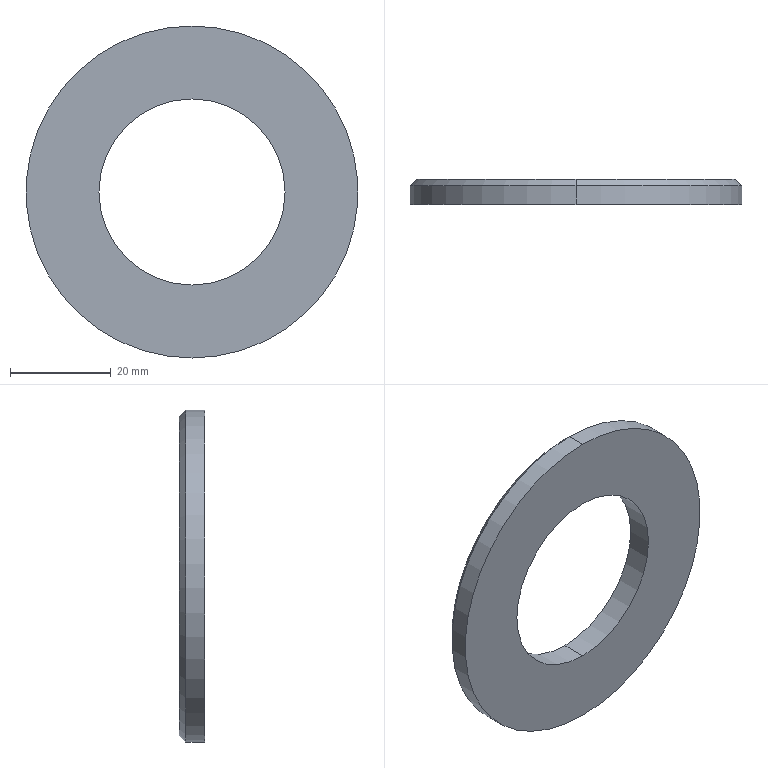Part | SolidWorks | features Revolution 1 | 1 solid | 8 faces | box 66 x 5 x 66 mm | volume 11570 mm3 | cylinder 4 | cone 2 | plane 2 | commonest cylinder face diameters 37 x2 66 x2
STEP:
#1=CARTESIAN_POINT('',(0.,12.395,-33.));
#2=VERTEX_POINT('',#1);
#3=CARTESIAN_POINT('',(0.,12.395,33.));
#4=VERTEX_POINT('',#3);
#5=CARTESIAN_POINT('',(0.,12.395,0.));
#6=DIRECTION('',(0.,-1.,0.));
#7=DIRECTION('',(0.,0.,-1.));
#8=AXIS2_PLACEMENT_3D('',#5,#6,#7);
#9=CIRCLE('',#8,33.);
#10=EDGE_CURVE('',#2,#4,#9,.T.);
#11=ORIENTED_EDGE('',*,*,#10,.T.);
#12=CARTESIAN_POINT('',(0.,8.645,33.));
#13=VERTEX_POINT('',#12);
#14=CARTESIAN_POINT('',(0.,0.,33.));
#15=DIRECTION('',(0.,-1.,0.));
#16=VECTOR('',#15,1000.);
#17=LINE('',#14,#16);
#18=EDGE_CURVE('',#4,#13,#17,.T.);
#19=ORIENTED_EDGE('',*,*,#18,.T.);
#20=CARTESIAN_POINT('',(0.,8.645,-33.));
#21=VERTEX_POINT('',#20);
#22=CARTESIAN_POINT('',(0.,8.645,0.));
#23=DIRECTION('',(0.,-1.,0.));
#24=DIRECTION('',(0.,0.,-1.));
#25=AXIS2_PLACEMENT_3D('',#22,#23,#24);
#26=CIRCLE('',#25,33.);
#27=EDGE_CURVE('',#21,#13,#26,.T.);
#28=ORIENTED_EDGE('',*,*,#27,.F.);
#29=CARTESIAN_POINT('',(0.,0.,-33.));
#30=DIRECTION('',(0.,-1.,0.));
#31=VECTOR('',#30,1000.);
#32=LINE('',#29,#31);
#33=EDGE_CURVE('',#2,#21,#32,.T.);
#34=ORIENTED_EDGE('',*,*,#33,.F.);
#35=EDGE_LOOP('',(#11,#19,#28,#34));
#36=FACE_OUTER_BOUND('',#35,.T.);
#37=CARTESIAN_POINT('',(0.,0.,0.));
#38=DIRECTION('',(0.,-1.,0.));
#39=DIRECTION('',(0.,0.,-1.));
#40=AXIS2_PLACEMENT_3D('',#37,#38,#39);
#41=CYLINDRICAL_SURFACE('',#40,33.);
#42=ADVANCED_FACE('',(#36),#41,.T.);
#43=CARTESIAN_POINT('',(0.,13.645,-31.75));
#44=VERTEX_POINT('',#43);
#45=CARTESIAN_POINT('',(0.,13.645,31.75));
#46=VERTEX_POINT('',#45);
#47=CARTESIAN_POINT('',(0.,13.645,0.));
#48=DIRECTION('',(0.,-1.,0.));
#49=DIRECTION('',(0.,0.,-1.));
#50=AXIS2_PLACEMENT_3D('',#47,#48,#49);
#51=CIRCLE('',#50,31.75);
#52=EDGE_CURVE('',#44,#46,#51,.T.);
#53=ORIENTED_EDGE('',*,*,#52,.T.);
#54=CARTESIAN_POINT('',(0.,13.645,31.75));
#55=DIRECTION('',(0.,-0.7071,0.7071));
#56=VECTOR('',#55,1000.);
#57=LINE('',#54,#56);
#58=EDGE_CURVE('',#46,#4,#57,.T.);
#59=ORIENTED_EDGE('',*,*,#58,.T.);
#60=ORIENTED_EDGE('',*,*,#10,.F.);
#61=CARTESIAN_POINT('',(0.,13.645,-31.75));
#62=DIRECTION('',(0.,-0.7071,-0.7071));
#63=VECTOR('',#62,1000.);
#64=LINE('',#61,#63);
#65=EDGE_CURVE('',#44,#2,#64,.T.);
#66=ORIENTED_EDGE('',*,*,#65,.F.);
#67=EDGE_LOOP('',(#53,#59,#60,#66));
#68=FACE_OUTER_BOUND('',#67,.T.);
#69=CARTESIAN_POINT('',(0.,13.645,0.));
#70=DIRECTION('',(0.,-1.,0.));
#71=DIRECTION('',(0.,0.,-1.));
#72=AXIS2_PLACEMENT_3D('',#69,#70,#71);
#73=CONICAL_SURFACE('',#72,31.75,0.7854);
#74=ADVANCED_FACE('',(#68),#73,.T.);
#75=CARTESIAN_POINT('',(0.,13.645,18.5));
#76=VERTEX_POINT('',#75);
#77=CARTESIAN_POINT('',(0.,13.645,-18.5));
#78=VERTEX_POINT('',#77);
#79=CARTESIAN_POINT('',(0.,13.645,0.));
#80=DIRECTION('',(0.,-1.,0.));
#81=DIRECTION('',(0.,0.,-1.));
#82=AXIS2_PLACEMENT_3D('',#79,#80,#81);
#83=CIRCLE('',#82,18.5);
#84=EDGE_CURVE('',#76,#78,#83,.T.);
#85=ORIENTED_EDGE('',*,*,#84,.F.);
#86=CARTESIAN_POINT('',(0.,8.645,18.5));
#87=VERTEX_POINT('',#86);
#88=CARTESIAN_POINT('',(0.,0.,18.5));
#89=DIRECTION('',(0.,-1.,0.));
#90=VECTOR('',#89,1000.);
#91=LINE('',#88,#90);
#92=EDGE_CURVE('',#76,#87,#91,.T.);
#93=ORIENTED_EDGE('',*,*,#92,.T.);
#94=CARTESIAN_POINT('',(0.,8.645,-18.5));
#95=VERTEX_POINT('',#94);
#96=CARTESIAN_POINT('',(0.,8.645,0.));
#97=DIRECTION('',(0.,-1.,0.));
#98=DIRECTION('',(0.,0.,-1.));
#99=AXIS2_PLACEMENT_3D('',#96,#97,#98);
#100=CIRCLE('',#99,18.5);
#101=EDGE_CURVE('',#87,#95,#100,.T.);
#102=ORIENTED_EDGE('',*,*,#101,.T.);
#103=CARTESIAN_POINT('',(0.,0.,-18.5));
#104=DIRECTION('',(0.,-1.,0.));
#105=VECTOR('',#104,1000.);
#106=LINE('',#103,#105);
#107=EDGE_CURVE('',#78,#95,#106,.T.);
#108=ORIENTED_EDGE('',*,*,#107,.F.);
#109=EDGE_LOOP('',(#85,#93,#102,#108));
#110=FACE_OUTER_BOUND('',#109,.T.);
#111=CARTESIAN_POINT('',(0.,0.,0.));
#112=DIRECTION('',(0.,-1.,0.));
#113=DIRECTION('',(0.,0.,-1.));
#114=AXIS2_PLACEMENT_3D('',#111,#112,#113);
#115=CYLINDRICAL_SURFACE('',#114,18.5);
#116=ADVANCED_FACE('',(#110),#115,.F.);
#117=ORIENTED_EDGE('',*,*,#92,.F.);
#118=CARTESIAN_POINT('',(0.,13.645,0.));
#119=DIRECTION('',(0.,-1.,0.));
#120=DIRECTION('',(0.,0.,-1.));
#121=AXIS2_PLACEMENT_3D('',#118,#119,#120);
#122=CIRCLE('',#121,18.5);
#123=EDGE_CURVE('',#78,#76,#122,.T.);
#124=ORIENTED_EDGE('',*,*,#123,.F.);
#125=ORIENTED_EDGE('',*,*,#107,.T.);
#126=CARTESIAN_POINT('',(0.,8.645,0.));
#127=DIRECTION('',(0.,-1.,0.));
#128=DIRECTION('',(0.,0.,-1.));
#129=AXIS2_PLACEMENT_3D('',#126,#127,#128);
#130=CIRCLE('',#129,18.5);
#131=EDGE_CURVE('',#95,#87,#130,.T.);
#132=ORIENTED_EDGE('',*,*,#131,.T.);
#133=EDGE_LOOP('',(#117,#124,#125,#132));
#134=FACE_OUTER_BOUND('',#133,.T.);
#135=CARTESIAN_POINT('',(0.,0.,0.));
#136=DIRECTION('',(0.,-1.,0.));
#137=DIRECTION('',(0.,0.,-1.));
#138=AXIS2_PLACEMENT_3D('',#135,#136,#137);
#139=CYLINDRICAL_SURFACE('',#138,18.5);
#140=ADVANCED_FACE('',(#134),#139,.F.);
#141=ORIENTED_EDGE('',*,*,#52,.F.);
#142=CARTESIAN_POINT('',(0.,13.645,0.));
#143=DIRECTION('',(0.,-1.,0.));
#144=DIRECTION('',(0.,0.,-1.));
#145=AXIS2_PLACEMENT_3D('',#142,#143,#144);
#146=CIRCLE('',#145,31.75);
#147=EDGE_CURVE('',#46,#44,#146,.T.);
#148=ORIENTED_EDGE('',*,*,#147,.F.);
#149=EDGE_LOOP('',(#141,#148));
#150=FACE_OUTER_BOUND('',#149,.T.);
#151=ORIENTED_EDGE('',*,*,#123,.T.);
#152=ORIENTED_EDGE('',*,*,#84,.T.);
#153=EDGE_LOOP('',(#151,#152));
#154=FACE_BOUND('',#153,.T.);
#155=CARTESIAN_POINT('',(-18.5,13.645,0.));
#156=DIRECTION('',(0.,-1.,0.));
#157=DIRECTION('',(0.,0.,-1.));
#158=AXIS2_PLACEMENT_3D('',#155,#156,#157);
#159=PLANE('',#158);
#160=ADVANCED_FACE('',(#150,#154),#159,.F.);
#161=ORIENTED_EDGE('',*,*,#58,.F.);
#162=ORIENTED_EDGE('',*,*,#147,.T.);
#163=ORIENTED_EDGE('',*,*,#65,.T.);
#164=CARTESIAN_POINT('',(0.,12.395,0.));
#165=DIRECTION('',(0.,-1.,0.));
#166=DIRECTION('',(0.,0.,-1.));
#167=AXIS2_PLACEMENT_3D('',#164,#165,#166);
#168=CIRCLE('',#167,33.);
#169=EDGE_CURVE('',#4,#2,#168,.T.);
#170=ORIENTED_EDGE('',*,*,#169,.F.);
#171=EDGE_LOOP('',(#161,#162,#163,#170));
#172=FACE_OUTER_BOUND('',#171,.T.);
#173=CARTESIAN_POINT('',(0.,13.645,0.));
#174=DIRECTION('',(0.,-1.,0.));
#175=DIRECTION('',(0.,0.,-1.));
#176=AXIS2_PLACEMENT_3D('',#173,#174,#175);
#177=CONICAL_SURFACE('',#176,31.75,0.7854);
#178=ADVANCED_FACE('',(#172),#177,.T.);
#179=ORIENTED_EDGE('',*,*,#18,.F.);
#180=ORIENTED_EDGE('',*,*,#169,.T.);
#181=ORIENTED_EDGE('',*,*,#33,.T.);
#182=CARTESIAN_POINT('',(0.,8.645,0.));
#183=DIRECTION('',(0.,-1.,0.));
#184=DIRECTION('',(0.,0.,-1.));
#185=AXIS2_PLACEMENT_3D('',#182,#183,#184);
#186=CIRCLE('',#185,33.);
#187=EDGE_CURVE('',#13,#21,#186,.T.);
#188=ORIENTED_EDGE('',*,*,#187,.F.);
#189=EDGE_LOOP('',(#179,#180,#181,#188));
#190=FACE_OUTER_BOUND('',#189,.T.);
#191=CARTESIAN_POINT('',(0.,0.,0.));
#192=DIRECTION('',(0.,-1.,0.));
#193=DIRECTION('',(0.,0.,-1.));
#194=AXIS2_PLACEMENT_3D('',#191,#192,#193);
#195=CYLINDRICAL_SURFACE('',#194,33.);
#196=ADVANCED_FACE('',(#190),#195,.T.);
#197=ORIENTED_EDGE('',*,*,#131,.F.);
#198=ORIENTED_EDGE('',*,*,#101,.F.);
#199=EDGE_LOOP('',(#197,#198));
#200=FACE_BOUND('',#199,.T.);
#201=ORIENTED_EDGE('',*,*,#27,.T.);
#202=ORIENTED_EDGE('',*,*,#187,.T.);
#203=EDGE_LOOP('',(#201,#202));
#204=FACE_OUTER_BOUND('',#203,.T.);
#205=CARTESIAN_POINT('',(-18.5,8.645,0.));
#206=DIRECTION('',(0.,1.,0.));
#207=DIRECTION('',(0.,0.,1.));
#208=AXIS2_PLACEMENT_3D('',#205,#206,#207);
#209=PLANE('',#208);
#210=ADVANCED_FACE('',(#200,#204),#209,.F.);
#211=CLOSED_SHELL('',(#42,#74,#116,#140,#160,#178,#196,#210));
#212=MANIFOLD_SOLID_BREP('',#211);
#213=CARTESIAN_POINT('',(0.,0.,0.));
#214=DIRECTION('',(0.,0.,1.));
#215=DIRECTION('',(1.,0.,0.));
#216=AXIS2_PLACEMENT_3D('',#213,#214,#215);
#217=(LENGTH_UNIT()NAMED_UNIT(*)SI_UNIT(.MILLI.,.METRE.));
#218=UNCERTAINTY_MEASURE_WITH_UNIT(LENGTH_MEASURE(0.00001),#217,'','');
#219=(NAMED_UNIT(*)PLANE_ANGLE_UNIT()SI_UNIT($,.RADIAN.));
#220=(NAMED_UNIT(*)SI_UNIT($,.STERADIAN.)SOLID_ANGLE_UNIT());
#221=(GEOMETRIC_REPRESENTATION_CONTEXT(3)GLOBAL_UNCERTAINTY_ASSIGNED_CONTEXT((#218))GLOBAL_UNIT_ASSIGNED_CONTEXT((#217,#219,#220))REPRESENTATION_CONTEXT('',''));
#222=ADVANCED_BREP_SHAPE_REPRESENTATION('',(#212,#216),#221);